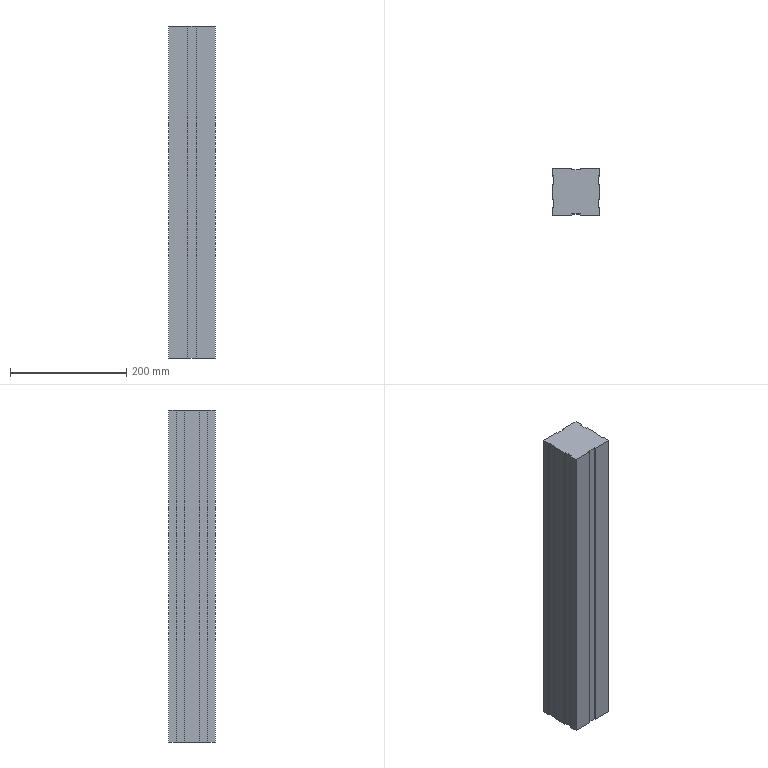Part | STEP file | xingcai80x80x570 | 1 solid | 30 faces | box 80 x 80 x 570 mm | volume 3552240 mm3 | plane 30